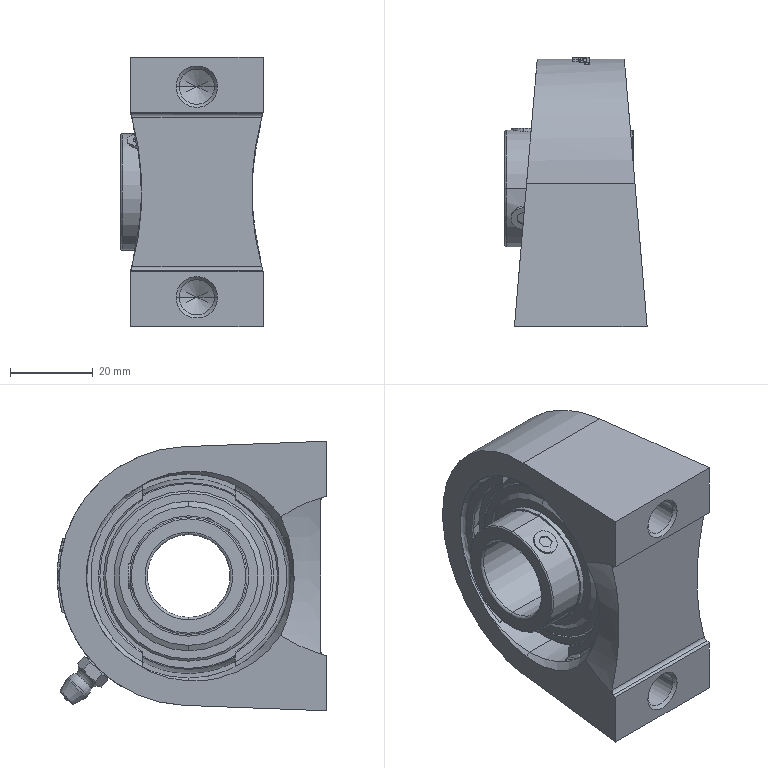Part | SolidWorks | features AEMSimFeature 1 | 11 solids | 432 faces | box 34.3 x 65 x 65 mm | volume 66950 mm3 | plane 133 | cylinder 124 | cone 97 | torus 52 | sphere 26 | commonest cylinder face diameters 0.129 x14 0.222 x14 28.2 x14 0.41 x13 0.126 x10 2 x4